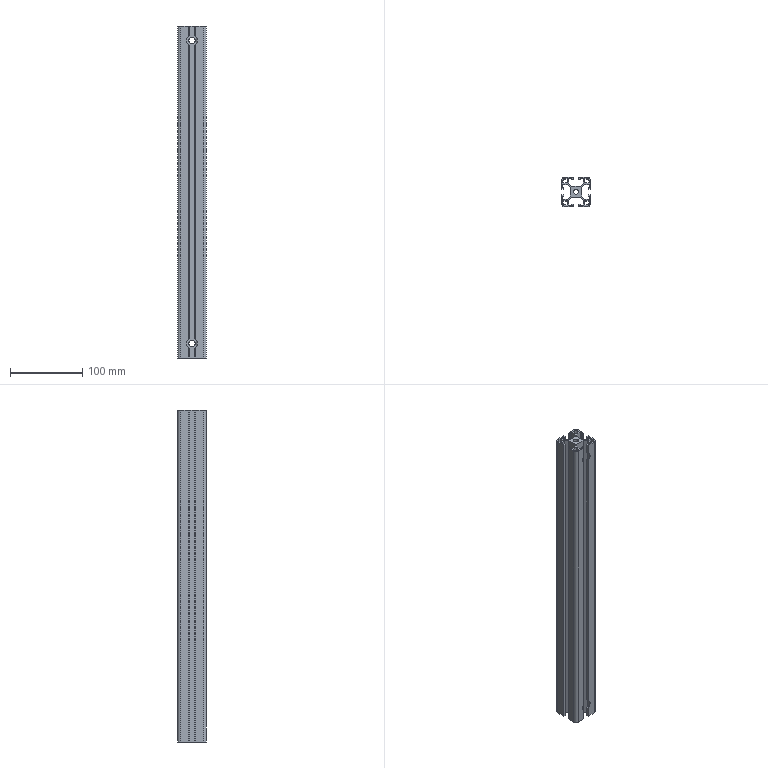Part | STEP file | 1 solid | 144 faces | box 40 x 40 x 458 mm | volume 262404 mm3 | plane 118 | cylinder 26 | commonest cylinder face diameters 9 x12 6.8 x6 5 x4 15 x4